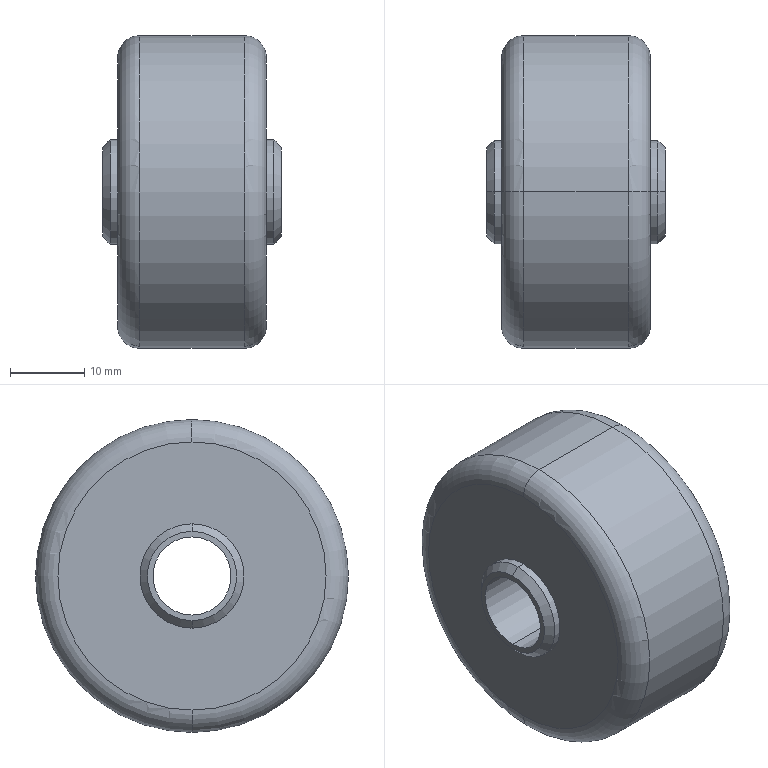Part | NX | features BREP 1 | 1 solid | 20 faces | box 24 x 42 x 42 mm | volume 25711 mm3 | cylinder 8 | torus 4 | cone 4 | plane 4 | commonest cylinder face diameters 14 x4 10.5 x2 42 x2
STEP:
#1=CARTESIAN_POINT('',(-10.,0.,7.));
#2=VERTEX_POINT('',#1);
#3=CARTESIAN_POINT('',(-10.,0.,-7.));
#4=VERTEX_POINT('',#3);
#5=CARTESIAN_POINT('',(-10.,0.,0.));
#6=DIRECTION('',(1.,0.,0.));
#7=DIRECTION('',(0.,0.,-1.));
#8=AXIS2_PLACEMENT_3D('',#5,#6,#7);
#9=CIRCLE('',#8,7.);
#10=EDGE_CURVE('',#2,#4,#9,.T.);
#11=ORIENTED_EDGE('',*,*,#10,.F.);
#12=CARTESIAN_POINT('',(-11.,0.,7.));
#13=VERTEX_POINT('',#12);
#14=CARTESIAN_POINT('',(50.,0.,7.));
#15=DIRECTION('',(-1.,0.,0.));
#16=VECTOR('',#15,1000.);
#17=LINE('',#14,#16);
#18=EDGE_CURVE('',#2,#13,#17,.T.);
#19=ORIENTED_EDGE('',*,*,#18,.T.);
#20=CARTESIAN_POINT('',(-11.,0.,-7.));
#21=VERTEX_POINT('',#20);
#22=CARTESIAN_POINT('',(-11.,0.,0.));
#23=DIRECTION('',(1.,0.,0.));
#24=DIRECTION('',(0.,0.,-1.));
#25=AXIS2_PLACEMENT_3D('',#22,#23,#24);
#26=CIRCLE('',#25,7.);
#27=EDGE_CURVE('',#13,#21,#26,.T.);
#28=ORIENTED_EDGE('',*,*,#27,.T.);
#29=CARTESIAN_POINT('',(50.,0.,-7.));
#30=DIRECTION('',(-1.,0.,0.));
#31=VECTOR('',#30,1000.);
#32=LINE('',#29,#31);
#33=EDGE_CURVE('',#4,#21,#32,.T.);
#34=ORIENTED_EDGE('',*,*,#33,.F.);
#35=EDGE_LOOP('',(#11,#19,#28,#34));
#36=FACE_BOUND('',#35,.T.);
#37=CARTESIAN_POINT('',(50.,0.,0.));
#38=DIRECTION('',(-1.,0.,0.));
#39=DIRECTION('',(0.,0.,-1.));
#40=AXIS2_PLACEMENT_3D('',#37,#38,#39);
#41=CYLINDRICAL_SURFACE('',#40,7.);
#42=ADVANCED_FACE('',(#36),#41,.T.);
#43=CARTESIAN_POINT('',(-10.,0.,-18.));
#44=VERTEX_POINT('',#43);
#45=CARTESIAN_POINT('',(-10.,0.,18.));
#46=VERTEX_POINT('',#45);
#47=CARTESIAN_POINT('',(-10.,0.,0.));
#48=DIRECTION('',(1.,0.,0.));
#49=DIRECTION('',(0.,0.,-1.));
#50=AXIS2_PLACEMENT_3D('',#47,#48,#49);
#51=CIRCLE('',#50,18.);
#52=EDGE_CURVE('',#44,#46,#51,.T.);
#53=ORIENTED_EDGE('',*,*,#52,.T.);
#54=CARTESIAN_POINT('',(-7.,0.,21.));
#55=VERTEX_POINT('',#54);
#56=CARTESIAN_POINT('',(-7.,0.,18.));
#57=DIRECTION('',(0.,1.,0.));
#58=DIRECTION('',(0.,0.,1.));
#59=AXIS2_PLACEMENT_3D('',#56,#57,#58);
#60=CIRCLE('',#59,3.);
#61=EDGE_CURVE('',#46,#55,#60,.T.);
#62=ORIENTED_EDGE('',*,*,#61,.T.);
#63=CARTESIAN_POINT('',(-7.,0.,-21.));
#64=VERTEX_POINT('',#63);
#65=CARTESIAN_POINT('',(-7.,0.,0.));
#66=DIRECTION('',(1.,0.,0.));
#67=DIRECTION('',(0.,0.,-1.));
#68=AXIS2_PLACEMENT_3D('',#65,#66,#67);
#69=CIRCLE('',#68,21.);
#70=EDGE_CURVE('',#64,#55,#69,.T.);
#71=ORIENTED_EDGE('',*,*,#70,.F.);
#72=CARTESIAN_POINT('',(-7.,0.,-18.));
#73=DIRECTION('',(0.,-1.,0.));
#74=DIRECTION('',(0.,0.,-1.));
#75=AXIS2_PLACEMENT_3D('',#72,#73,#74);
#76=CIRCLE('',#75,3.);
#77=EDGE_CURVE('',#44,#64,#76,.T.);
#78=ORIENTED_EDGE('',*,*,#77,.F.);
#79=EDGE_LOOP('',(#53,#62,#71,#78));
#80=FACE_BOUND('',#79,.T.);
#81=CARTESIAN_POINT('',(-7.,0.,0.));
#82=DIRECTION('',(1.,0.,0.));
#83=DIRECTION('',(0.,0.,-1.));
#84=AXIS2_PLACEMENT_3D('',#81,#82,#83);
#85=TOROIDAL_SURFACE('',#84,18.,3.);
#86=ADVANCED_FACE('',(#80),#85,.T.);
#87=CARTESIAN_POINT('',(7.,0.,21.));
#88=VERTEX_POINT('',#87);
#89=CARTESIAN_POINT('',(7.,0.,-21.));
#90=VERTEX_POINT('',#89);
#91=CARTESIAN_POINT('',(7.,0.,0.));
#92=DIRECTION('',(1.,0.,0.));
#93=DIRECTION('',(0.,0.,-1.));
#94=AXIS2_PLACEMENT_3D('',#91,#92,#93);
#95=CIRCLE('',#94,21.);
#96=EDGE_CURVE('',#88,#90,#95,.T.);
#97=ORIENTED_EDGE('',*,*,#96,.F.);
#98=CARTESIAN_POINT('',(50.,0.,21.));
#99=DIRECTION('',(-1.,0.,0.));
#100=VECTOR('',#99,1000.);
#101=LINE('',#98,#100);
#102=EDGE_CURVE('',#88,#55,#101,.T.);
#103=ORIENTED_EDGE('',*,*,#102,.T.);
#104=CARTESIAN_POINT('',(-7.,0.,0.));
#105=DIRECTION('',(1.,0.,0.));
#106=DIRECTION('',(0.,0.,-1.));
#107=AXIS2_PLACEMENT_3D('',#104,#105,#106);
#108=CIRCLE('',#107,21.);
#109=EDGE_CURVE('',#55,#64,#108,.T.);
#110=ORIENTED_EDGE('',*,*,#109,.T.);
#111=CARTESIAN_POINT('',(50.,0.,-21.));
#112=DIRECTION('',(-1.,0.,0.));
#113=VECTOR('',#112,1000.);
#114=LINE('',#111,#113);
#115=EDGE_CURVE('',#90,#64,#114,.T.);
#116=ORIENTED_EDGE('',*,*,#115,.F.);
#117=EDGE_LOOP('',(#97,#103,#110,#116));
#118=FACE_BOUND('',#117,.T.);
#119=CARTESIAN_POINT('',(50.,0.,0.));
#120=DIRECTION('',(-1.,0.,0.));
#121=DIRECTION('',(0.,0.,-1.));
#122=AXIS2_PLACEMENT_3D('',#119,#120,#121);
#123=CYLINDRICAL_SURFACE('',#122,21.);
#124=ADVANCED_FACE('',(#118),#123,.T.);
#125=CARTESIAN_POINT('',(7.,0.,0.));
#126=DIRECTION('',(1.,0.,0.));
#127=DIRECTION('',(0.,0.,-1.));
#128=AXIS2_PLACEMENT_3D('',#125,#126,#127);
#129=CIRCLE('',#128,21.);
#130=EDGE_CURVE('',#90,#88,#129,.T.);
#131=ORIENTED_EDGE('',*,*,#130,.T.);
#132=CARTESIAN_POINT('',(10.,0.,18.));
#133=VERTEX_POINT('',#132);
#134=CARTESIAN_POINT('',(7.,0.,18.));
#135=DIRECTION('',(0.,1.,0.));
#136=DIRECTION('',(0.,0.,1.));
#137=AXIS2_PLACEMENT_3D('',#134,#135,#136);
#138=CIRCLE('',#137,3.);
#139=EDGE_CURVE('',#88,#133,#138,.T.);
#140=ORIENTED_EDGE('',*,*,#139,.T.);
#141=CARTESIAN_POINT('',(10.,0.,-18.));
#142=VERTEX_POINT('',#141);
#143=CARTESIAN_POINT('',(10.,0.,0.));
#144=DIRECTION('',(1.,0.,0.));
#145=DIRECTION('',(0.,0.,-1.));
#146=AXIS2_PLACEMENT_3D('',#143,#144,#145);
#147=CIRCLE('',#146,18.);
#148=EDGE_CURVE('',#142,#133,#147,.T.);
#149=ORIENTED_EDGE('',*,*,#148,.F.);
#150=CARTESIAN_POINT('',(7.,0.,-18.));
#151=DIRECTION('',(0.,-1.,0.));
#152=DIRECTION('',(0.,0.,-1.));
#153=AXIS2_PLACEMENT_3D('',#150,#151,#152);
#154=CIRCLE('',#153,3.);
#155=EDGE_CURVE('',#90,#142,#154,.T.);
#156=ORIENTED_EDGE('',*,*,#155,.F.);
#157=EDGE_LOOP('',(#131,#140,#149,#156));
#158=FACE_BOUND('',#157,.T.);
#159=CARTESIAN_POINT('',(7.,0.,0.));
#160=DIRECTION('',(1.,0.,0.));
#161=DIRECTION('',(0.,0.,-1.));
#162=AXIS2_PLACEMENT_3D('',#159,#160,#161);
#163=TOROIDAL_SURFACE('',#162,18.,3.);
#164=ADVANCED_FACE('',(#158),#163,.T.);
#165=CARTESIAN_POINT('',(11.,0.,7.));
#166=VERTEX_POINT('',#165);
#167=CARTESIAN_POINT('',(11.,0.,-7.));
#168=VERTEX_POINT('',#167);
#169=CARTESIAN_POINT('',(11.,0.,0.));
#170=DIRECTION('',(1.,0.,0.));
#171=DIRECTION('',(0.,0.,-1.));
#172=AXIS2_PLACEMENT_3D('',#169,#170,#171);
#173=CIRCLE('',#172,7.);
#174=EDGE_CURVE('',#166,#168,#173,.T.);
#175=ORIENTED_EDGE('',*,*,#174,.F.);
#176=CARTESIAN_POINT('',(10.,0.,7.));
#177=VERTEX_POINT('',#176);
#178=CARTESIAN_POINT('',(50.,0.,7.));
#179=DIRECTION('',(-1.,0.,0.));
#180=VECTOR('',#179,1000.);
#181=LINE('',#178,#180);
#182=EDGE_CURVE('',#166,#177,#181,.T.);
#183=ORIENTED_EDGE('',*,*,#182,.T.);
#184=CARTESIAN_POINT('',(10.,0.,-7.));
#185=VERTEX_POINT('',#184);
#186=CARTESIAN_POINT('',(10.,0.,0.));
#187=DIRECTION('',(1.,0.,0.));
#188=DIRECTION('',(0.,0.,-1.));
#189=AXIS2_PLACEMENT_3D('',#186,#187,#188);
#190=CIRCLE('',#189,7.);
#191=EDGE_CURVE('',#177,#185,#190,.T.);
#192=ORIENTED_EDGE('',*,*,#191,.T.);
#193=CARTESIAN_POINT('',(50.,0.,-7.));
#194=DIRECTION('',(-1.,0.,0.));
#195=VECTOR('',#194,1000.);
#196=LINE('',#193,#195);
#197=EDGE_CURVE('',#168,#185,#196,.T.);
#198=ORIENTED_EDGE('',*,*,#197,.F.);
#199=EDGE_LOOP('',(#175,#183,#192,#198));
#200=FACE_BOUND('',#199,.T.);
#201=CARTESIAN_POINT('',(50.,0.,0.));
#202=DIRECTION('',(-1.,0.,0.));
#203=DIRECTION('',(0.,0.,-1.));
#204=AXIS2_PLACEMENT_3D('',#201,#202,#203);
#205=CYLINDRICAL_SURFACE('',#204,7.);
#206=ADVANCED_FACE('',(#200),#205,.T.);
#207=CARTESIAN_POINT('',(12.,0.,-6.));
#208=VERTEX_POINT('',#207);
#209=CARTESIAN_POINT('',(12.,0.,6.));
#210=VERTEX_POINT('',#209);
#211=CARTESIAN_POINT('',(12.,0.,0.));
#212=DIRECTION('',(1.,0.,0.));
#213=DIRECTION('',(0.,0.,-1.));
#214=AXIS2_PLACEMENT_3D('',#211,#212,#213);
#215=CIRCLE('',#214,6.);
#216=EDGE_CURVE('',#208,#210,#215,.T.);
#217=ORIENTED_EDGE('',*,*,#216,.F.);
#218=CARTESIAN_POINT('',(12.,0.,-6.));
#219=DIRECTION('',(-0.7071,0.,-0.7071));
#220=VECTOR('',#219,1000.);
#221=LINE('',#218,#220);
#222=EDGE_CURVE('',#168,#208,#221,.F.);
#223=ORIENTED_EDGE('',*,*,#222,.F.);
#224=CARTESIAN_POINT('',(11.,0.,0.));
#225=DIRECTION('',(1.,0.,0.));
#226=DIRECTION('',(0.,0.,-1.));
#227=AXIS2_PLACEMENT_3D('',#224,#225,#226);
#228=CIRCLE('',#227,7.);
#229=EDGE_CURVE('',#168,#166,#228,.T.);
#230=ORIENTED_EDGE('',*,*,#229,.T.);
#231=CARTESIAN_POINT('',(12.,0.,6.));
#232=DIRECTION('',(-0.7071,0.,0.7071));
#233=VECTOR('',#232,1000.);
#234=LINE('',#231,#233);
#235=EDGE_CURVE('',#166,#210,#234,.F.);
#236=ORIENTED_EDGE('',*,*,#235,.T.);
#237=EDGE_LOOP('',(#217,#223,#230,#236));
#238=FACE_BOUND('',#237,.T.);
#239=CARTESIAN_POINT('',(12.,0.,0.));
#240=DIRECTION('',(-1.,0.,0.));
#241=DIRECTION('',(0.,0.,1.));
#242=AXIS2_PLACEMENT_3D('',#239,#240,#241);
#243=CONICAL_SURFACE('',#242,6.,0.7854);
#244=ADVANCED_FACE('',(#238),#243,.T.);
#245=CARTESIAN_POINT('',(12.,0.,-5.25));
#246=VERTEX_POINT('',#245);
#247=CARTESIAN_POINT('',(12.,0.,5.25));
#248=VERTEX_POINT('',#247);
#249=CARTESIAN_POINT('',(12.,0.,0.));
#250=DIRECTION('',(1.,0.,0.));
#251=DIRECTION('',(0.,0.,-1.));
#252=AXIS2_PLACEMENT_3D('',#249,#250,#251);
#253=CIRCLE('',#252,5.25);
#254=EDGE_CURVE('',#246,#248,#253,.T.);
#255=ORIENTED_EDGE('',*,*,#254,.T.);
#256=CARTESIAN_POINT('',(-12.,0.,5.25));
#257=VERTEX_POINT('',#256);
#258=CARTESIAN_POINT('',(50.,0.,5.25));
#259=DIRECTION('',(-1.,0.,0.));
#260=VECTOR('',#259,1000.);
#261=LINE('',#258,#260);
#262=EDGE_CURVE('',#248,#257,#261,.T.);
#263=ORIENTED_EDGE('',*,*,#262,.T.);
#264=CARTESIAN_POINT('',(-12.,0.,-5.25));
#265=VERTEX_POINT('',#264);
#266=CARTESIAN_POINT('',(-12.,0.,0.));
#267=DIRECTION('',(1.,0.,0.));
#268=DIRECTION('',(0.,0.,-1.));
#269=AXIS2_PLACEMENT_3D('',#266,#267,#268);
#270=CIRCLE('',#269,5.25);
#271=EDGE_CURVE('',#265,#257,#270,.T.);
#272=ORIENTED_EDGE('',*,*,#271,.F.);
#273=CARTESIAN_POINT('',(50.,0.,-5.25));
#274=DIRECTION('',(-1.,0.,0.));
#275=VECTOR('',#274,1000.);
#276=LINE('',#273,#275);
#277=EDGE_CURVE('',#246,#265,#276,.T.);
#278=ORIENTED_EDGE('',*,*,#277,.F.);
#279=EDGE_LOOP('',(#255,#263,#272,#278));
#280=FACE_BOUND('',#279,.T.);
#281=CARTESIAN_POINT('',(50.,0.,0.));
#282=DIRECTION('',(-1.,0.,0.));
#283=DIRECTION('',(0.,0.,-1.));
#284=AXIS2_PLACEMENT_3D('',#281,#282,#283);
#285=CYLINDRICAL_SURFACE('',#284,5.25);
#286=ADVANCED_FACE('',(#280),#285,.F.);
#287=CARTESIAN_POINT('',(-12.,0.,-6.));
#288=VERTEX_POINT('',#287);
#289=CARTESIAN_POINT('',(-12.,0.,6.));
#290=VERTEX_POINT('',#289);
#291=CARTESIAN_POINT('',(-12.,0.,0.));
#292=DIRECTION('',(1.,0.,0.));
#293=DIRECTION('',(0.,0.,-1.));
#294=AXIS2_PLACEMENT_3D('',#291,#292,#293);
#295=CIRCLE('',#294,6.);
#296=EDGE_CURVE('',#288,#290,#295,.T.);
#297=ORIENTED_EDGE('',*,*,#296,.T.);
#298=CARTESIAN_POINT('',(-11.,0.,7.));
#299=DIRECTION('',(0.7071,0.,0.7071));
#300=VECTOR('',#299,1000.);
#301=LINE('',#298,#300);
#302=EDGE_CURVE('',#290,#13,#301,.T.);
#303=ORIENTED_EDGE('',*,*,#302,.T.);
#304=CARTESIAN_POINT('',(-11.,0.,0.));
#305=DIRECTION('',(1.,0.,0.));
#306=DIRECTION('',(0.,0.,-1.));
#307=AXIS2_PLACEMENT_3D('',#304,#305,#306);
#308=CIRCLE('',#307,7.);
#309=EDGE_CURVE('',#21,#13,#308,.T.);
#310=ORIENTED_EDGE('',*,*,#309,.F.);
#311=CARTESIAN_POINT('',(-11.,0.,-7.));
#312=DIRECTION('',(0.7071,0.,-0.7071));
#313=VECTOR('',#312,1000.);
#314=LINE('',#311,#313);
#315=EDGE_CURVE('',#288,#21,#314,.T.);
#316=ORIENTED_EDGE('',*,*,#315,.F.);
#317=EDGE_LOOP('',(#297,#303,#310,#316));
#318=FACE_BOUND('',#317,.T.);
#319=CARTESIAN_POINT('',(-11.,0.,0.));
#320=DIRECTION('',(1.,0.,0.));
#321=DIRECTION('',(0.,0.,-1.));
#322=AXIS2_PLACEMENT_3D('',#319,#320,#321);
#323=CONICAL_SURFACE('',#322,7.,0.7854);
#324=ADVANCED_FACE('',(#318),#323,.T.);
#325=ORIENTED_EDGE('',*,*,#302,.F.);
#326=CARTESIAN_POINT('',(-12.,0.,0.));
#327=DIRECTION('',(1.,0.,0.));
#328=DIRECTION('',(0.,0.,-1.));
#329=AXIS2_PLACEMENT_3D('',#326,#327,#328);
#330=CIRCLE('',#329,6.);
#331=EDGE_CURVE('',#290,#288,#330,.T.);
#332=ORIENTED_EDGE('',*,*,#331,.T.);
#333=ORIENTED_EDGE('',*,*,#315,.T.);
#334=ORIENTED_EDGE('',*,*,#27,.F.);
#335=EDGE_LOOP('',(#325,#332,#333,#334));
#336=FACE_BOUND('',#335,.T.);
#337=CARTESIAN_POINT('',(-11.,0.,0.));
#338=DIRECTION('',(1.,0.,0.));
#339=DIRECTION('',(0.,0.,-1.));
#340=AXIS2_PLACEMENT_3D('',#337,#338,#339);
#341=CONICAL_SURFACE('',#340,7.,0.7854);
#342=ADVANCED_FACE('',(#336),#341,.T.);
#343=ORIENTED_EDGE('',*,*,#296,.F.);
#344=ORIENTED_EDGE('',*,*,#331,.F.);
#345=EDGE_LOOP('',(#343,#344));
#346=FACE_BOUND('',#345,.T.);
#347=ORIENTED_EDGE('',*,*,#271,.T.);
#348=CARTESIAN_POINT('',(-12.,0.,0.));
#349=DIRECTION('',(1.,0.,0.));
#350=DIRECTION('',(0.,0.,-1.));
#351=AXIS2_PLACEMENT_3D('',#348,#349,#350);
#352=CIRCLE('',#351,5.25);
#353=EDGE_CURVE('',#257,#265,#352,.T.);
#354=ORIENTED_EDGE('',*,*,#353,.T.);
#355=EDGE_LOOP('',(#347,#354));
#356=FACE_BOUND('',#355,.T.);
#357=CARTESIAN_POINT('',(-12.,6.,0.));
#358=DIRECTION('',(-1.,0.,0.));
#359=DIRECTION('',(0.,0.,1.));
#360=AXIS2_PLACEMENT_3D('',#357,#358,#359);
#361=PLANE('',#360);
#362=ADVANCED_FACE('',(#346,#356),#361,.T.);
#363=ORIENTED_EDGE('',*,*,#262,.F.);
#364=CARTESIAN_POINT('',(12.,0.,0.));
#365=DIRECTION('',(1.,0.,0.));
#366=DIRECTION('',(0.,0.,-1.));
#367=AXIS2_PLACEMENT_3D('',#364,#365,#366);
#368=CIRCLE('',#367,5.25);
#369=EDGE_CURVE('',#248,#246,#368,.T.);
#370=ORIENTED_EDGE('',*,*,#369,.T.);
#371=ORIENTED_EDGE('',*,*,#277,.T.);
#372=ORIENTED_EDGE('',*,*,#353,.F.);
#373=EDGE_LOOP('',(#363,#370,#371,#372));
#374=FACE_BOUND('',#373,.T.);
#375=CARTESIAN_POINT('',(50.,0.,0.));
#376=DIRECTION('',(-1.,0.,0.));
#377=DIRECTION('',(0.,0.,-1.));
#378=AXIS2_PLACEMENT_3D('',#375,#376,#377);
#379=CYLINDRICAL_SURFACE('',#378,5.25);
#380=ADVANCED_FACE('',(#374),#379,.F.);
#381=CARTESIAN_POINT('',(12.,0.,0.));
#382=DIRECTION('',(1.,0.,0.));
#383=DIRECTION('',(0.,0.,-1.));
#384=AXIS2_PLACEMENT_3D('',#381,#382,#383);
#385=CIRCLE('',#384,6.);
#386=EDGE_CURVE('',#210,#208,#385,.T.);
#387=ORIENTED_EDGE('',*,*,#386,.T.);
#388=ORIENTED_EDGE('',*,*,#216,.T.);
#389=EDGE_LOOP('',(#387,#388));
#390=FACE_BOUND('',#389,.T.);
#391=ORIENTED_EDGE('',*,*,#254,.F.);
#392=ORIENTED_EDGE('',*,*,#369,.F.);
#393=EDGE_LOOP('',(#391,#392));
#394=FACE_BOUND('',#393,.T.);
#395=CARTESIAN_POINT('',(12.,5.25,0.));
#396=DIRECTION('',(1.,0.,0.));
#397=DIRECTION('',(0.,1.,0.));
#398=AXIS2_PLACEMENT_3D('',#395,#396,#397);
#399=PLANE('',#398);
#400=ADVANCED_FACE('',(#390,#394),#399,.T.);
#401=ORIENTED_EDGE('',*,*,#222,.T.);
#402=ORIENTED_EDGE('',*,*,#386,.F.);
#403=ORIENTED_EDGE('',*,*,#235,.F.);
#404=ORIENTED_EDGE('',*,*,#174,.T.);
#405=EDGE_LOOP('',(#401,#402,#403,#404));
#406=FACE_BOUND('',#405,.T.);
#407=CARTESIAN_POINT('',(12.,0.,0.));
#408=DIRECTION('',(-1.,0.,0.));
#409=DIRECTION('',(0.,0.,1.));
#410=AXIS2_PLACEMENT_3D('',#407,#408,#409);
#411=CONICAL_SURFACE('',#410,6.,0.7854);
#412=ADVANCED_FACE('',(#406),#411,.T.);
#413=ORIENTED_EDGE('',*,*,#182,.F.);
#414=ORIENTED_EDGE('',*,*,#229,.F.);
#415=ORIENTED_EDGE('',*,*,#197,.T.);
#416=CARTESIAN_POINT('',(10.,0.,0.));
#417=DIRECTION('',(1.,0.,0.));
#418=DIRECTION('',(0.,0.,-1.));
#419=AXIS2_PLACEMENT_3D('',#416,#417,#418);
#420=CIRCLE('',#419,7.);
#421=EDGE_CURVE('',#185,#177,#420,.T.);
#422=ORIENTED_EDGE('',*,*,#421,.T.);
#423=EDGE_LOOP('',(#413,#414,#415,#422));
#424=FACE_BOUND('',#423,.T.);
#425=CARTESIAN_POINT('',(50.,0.,0.));
#426=DIRECTION('',(-1.,0.,0.));
#427=DIRECTION('',(0.,0.,-1.));
#428=AXIS2_PLACEMENT_3D('',#425,#426,#427);
#429=CYLINDRICAL_SURFACE('',#428,7.);
#430=ADVANCED_FACE('',(#424),#429,.T.);
#431=ORIENTED_EDGE('',*,*,#148,.T.);
#432=CARTESIAN_POINT('',(10.,0.,0.));
#433=DIRECTION('',(1.,0.,0.));
#434=DIRECTION('',(0.,0.,-1.));
#435=AXIS2_PLACEMENT_3D('',#432,#433,#434);
#436=CIRCLE('',#435,18.);
#437=EDGE_CURVE('',#133,#142,#436,.T.);
#438=ORIENTED_EDGE('',*,*,#437,.T.);
#439=EDGE_LOOP('',(#431,#438));
#440=FACE_BOUND('',#439,.T.);
#441=ORIENTED_EDGE('',*,*,#421,.F.);
#442=ORIENTED_EDGE('',*,*,#191,.F.);
#443=EDGE_LOOP('',(#441,#442));
#444=FACE_BOUND('',#443,.T.);
#445=CARTESIAN_POINT('',(10.,7.,0.));
#446=DIRECTION('',(1.,0.,0.));
#447=DIRECTION('',(0.,1.,0.));
#448=AXIS2_PLACEMENT_3D('',#445,#446,#447);
#449=PLANE('',#448);
#450=ADVANCED_FACE('',(#440,#444),#449,.T.);
#451=ORIENTED_EDGE('',*,*,#139,.F.);
#452=ORIENTED_EDGE('',*,*,#96,.T.);
#453=ORIENTED_EDGE('',*,*,#155,.T.);
#454=ORIENTED_EDGE('',*,*,#437,.F.);
#455=EDGE_LOOP('',(#451,#452,#453,#454));
#456=FACE_BOUND('',#455,.T.);
#457=CARTESIAN_POINT('',(7.,0.,0.));
#458=DIRECTION('',(1.,0.,0.));
#459=DIRECTION('',(0.,0.,-1.));
#460=AXIS2_PLACEMENT_3D('',#457,#458,#459);
#461=TOROIDAL_SURFACE('',#460,18.,3.);
#462=ADVANCED_FACE('',(#456),#461,.T.);
#463=ORIENTED_EDGE('',*,*,#102,.F.);
#464=ORIENTED_EDGE('',*,*,#130,.F.);
#465=ORIENTED_EDGE('',*,*,#115,.T.);
#466=ORIENTED_EDGE('',*,*,#70,.T.);
#467=EDGE_LOOP('',(#463,#464,#465,#466));
#468=FACE_BOUND('',#467,.T.);
#469=CARTESIAN_POINT('',(50.,0.,0.));
#470=DIRECTION('',(-1.,0.,0.));
#471=DIRECTION('',(0.,0.,-1.));
#472=AXIS2_PLACEMENT_3D('',#469,#470,#471);
#473=CYLINDRICAL_SURFACE('',#472,21.);
#474=ADVANCED_FACE('',(#468),#473,.T.);
#475=ORIENTED_EDGE('',*,*,#61,.F.);
#476=CARTESIAN_POINT('',(-10.,0.,0.));
#477=DIRECTION('',(1.,0.,0.));
#478=DIRECTION('',(0.,0.,-1.));
#479=AXIS2_PLACEMENT_3D('',#476,#477,#478);
#480=CIRCLE('',#479,18.);
#481=EDGE_CURVE('',#46,#44,#480,.T.);
#482=ORIENTED_EDGE('',*,*,#481,.T.);
#483=ORIENTED_EDGE('',*,*,#77,.T.);
#484=ORIENTED_EDGE('',*,*,#109,.F.);
#485=EDGE_LOOP('',(#475,#482,#483,#484));
#486=FACE_BOUND('',#485,.T.);
#487=CARTESIAN_POINT('',(-7.,0.,0.));
#488=DIRECTION('',(1.,0.,0.));
#489=DIRECTION('',(0.,0.,-1.));
#490=AXIS2_PLACEMENT_3D('',#487,#488,#489);
#491=TOROIDAL_SURFACE('',#490,18.,3.);
#492=ADVANCED_FACE('',(#486),#491,.T.);
#493=ORIENTED_EDGE('',*,*,#52,.F.);
#494=ORIENTED_EDGE('',*,*,#481,.F.);
#495=EDGE_LOOP('',(#493,#494));
#496=FACE_BOUND('',#495,.T.);
#497=CARTESIAN_POINT('',(-10.,0.,0.));
#498=DIRECTION('',(1.,0.,0.));
#499=DIRECTION('',(0.,0.,-1.));
#500=AXIS2_PLACEMENT_3D('',#497,#498,#499);
#501=CIRCLE('',#500,7.);
#502=EDGE_CURVE('',#4,#2,#501,.T.);
#503=ORIENTED_EDGE('',*,*,#502,.T.);
#504=ORIENTED_EDGE('',*,*,#10,.T.);
#505=EDGE_LOOP('',(#503,#504));
#506=FACE_BOUND('',#505,.T.);
#507=CARTESIAN_POINT('',(-10.,18.,0.));
#508=DIRECTION('',(-1.,0.,0.));
#509=DIRECTION('',(0.,0.,1.));
#510=AXIS2_PLACEMENT_3D('',#507,#508,#509);
#511=PLANE('',#510);
#512=ADVANCED_FACE('',(#496,#506),#511,.T.);
#513=ORIENTED_EDGE('',*,*,#18,.F.);
#514=ORIENTED_EDGE('',*,*,#502,.F.);
#515=ORIENTED_EDGE('',*,*,#33,.T.);
#516=ORIENTED_EDGE('',*,*,#309,.T.);
#517=EDGE_LOOP('',(#513,#514,#515,#516));
#518=FACE_BOUND('',#517,.T.);
#519=CARTESIAN_POINT('',(50.,0.,0.));
#520=DIRECTION('',(-1.,0.,0.));
#521=DIRECTION('',(0.,0.,-1.));
#522=AXIS2_PLACEMENT_3D('',#519,#520,#521);
#523=CYLINDRICAL_SURFACE('',#522,7.);
#524=ADVANCED_FACE('',(#518),#523,.T.);
#525=CLOSED_SHELL('',(#42,#86,#124,#164,#206,#244,#286,#324,#342,#362,#380,#400,#412,#430,#450,#462,#474,#492,#512,#524));
#526=MANIFOLD_SOLID_BREP('',#525);
#527=(LENGTH_UNIT()NAMED_UNIT(*)SI_UNIT(.MILLI.,.METRE.));
#528=UNCERTAINTY_MEASURE_WITH_UNIT(LENGTH_MEASURE(0.00001),#527,'','');
#529=(NAMED_UNIT(*)PLANE_ANGLE_UNIT()SI_UNIT($,.RADIAN.));
#530=(NAMED_UNIT(*)SI_UNIT($,.STERADIAN.)SOLID_ANGLE_UNIT());
#531=(GEOMETRIC_REPRESENTATION_CONTEXT(3)GLOBAL_UNCERTAINTY_ASSIGNED_CONTEXT((#528))GLOBAL_UNIT_ASSIGNED_CONTEXT((#527,#529,#530))REPRESENTATION_CONTEXT('',''));
#532=ADVANCED_BREP_SHAPE_REPRESENTATION('',(#526),#531);